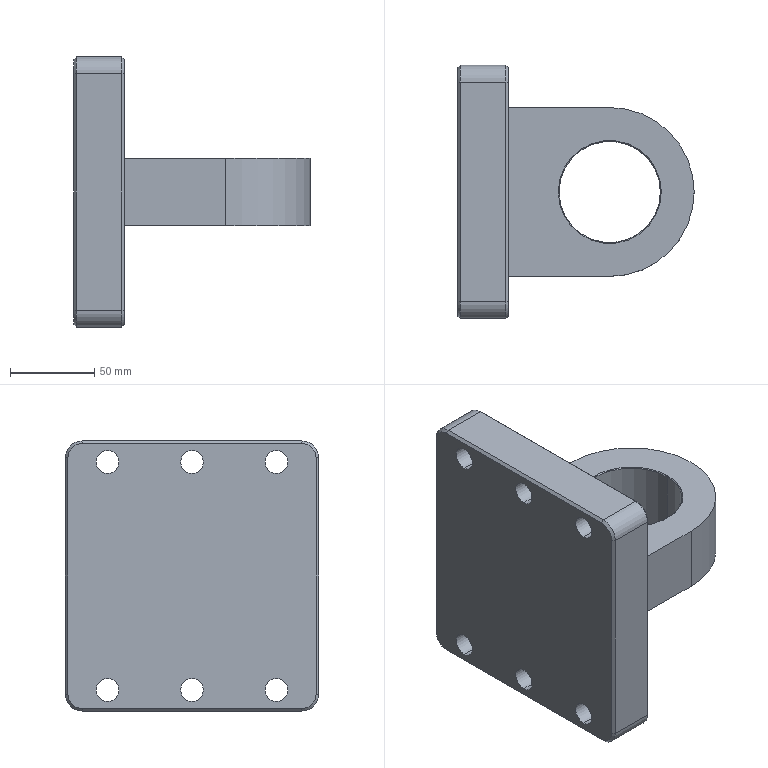Part | SolidWorks | features Chamfer 4, ICE 3, Fillet 2, Extrusion 1, HoleWzd 1, MirrorPattern 1 | 1 solid | 68 faces | box 140 x 150 x 160 mm | volume 960906 mm3 | cylinder 32 | plane 24 | cone 12 | commonest cylinder face diameters 20 x16 13.5 x12 60 x2 100 x2